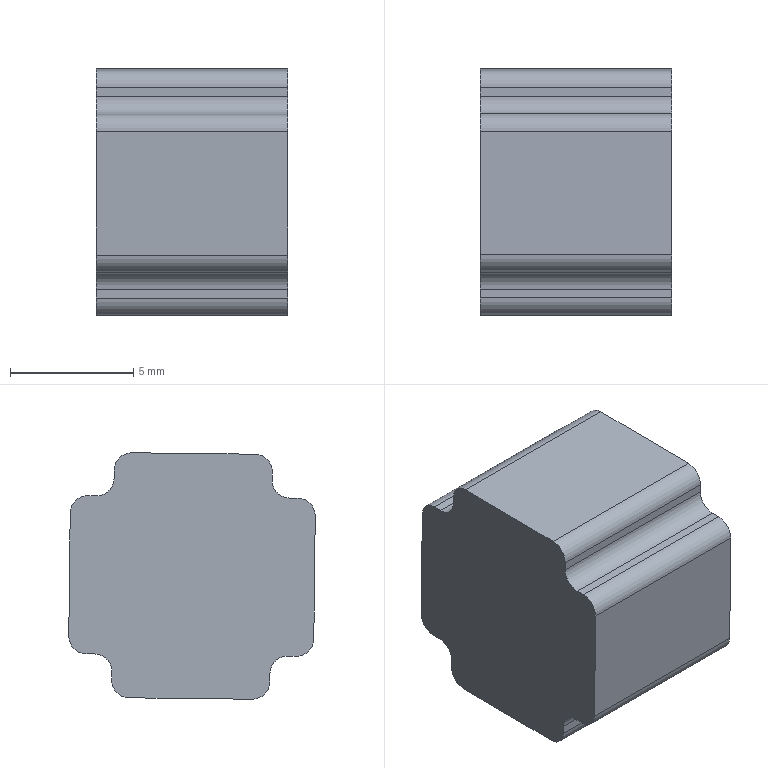Part | SolidWorks | features SplitBody 1 | 1 solid | 26 faces | box 7.744 x 9.983 x 9.983 mm | volume 663.797 mm3 | plane 14 | cylinder 12 | commonest cylinder face diameters 1.408 x12
STEP:
#1=CARTESIAN_POINT('',(576.371,440.454,-345.037));
#2=VERTEX_POINT('',#1);
#3=CARTESIAN_POINT('',(576.371,441.166,-345.733));
#4=VERTEX_POINT('',#3);
#5=CARTESIAN_POINT('',(576.371,441.158,-345.029));
#6=DIRECTION('',(1.,0.,0.));
#7=DIRECTION('',(0.,0.9999,0.01138));
#8=AXIS2_PLACEMENT_3D('',#5,#6,#7);
#9=CIRCLE('',#8,0.704);
#10=EDGE_CURVE('',#2,#4,#9,.T.);
#11=ORIENTED_EDGE('',*,*,#10,.T.);
#12=CARTESIAN_POINT('',(584.115,441.166,-345.733));
#13=VERTEX_POINT('',#12);
#14=CARTESIAN_POINT('',(584.115,441.166,-345.733));
#15=DIRECTION('',(-1.,0.,0.));
#16=VECTOR('',#15,1000.);
#17=LINE('',#14,#16);
#18=EDGE_CURVE('',#13,#4,#17,.T.);
#19=ORIENTED_EDGE('',*,*,#18,.F.);
#20=CARTESIAN_POINT('',(584.115,440.454,-345.037));
#21=VERTEX_POINT('',#20);
#22=CARTESIAN_POINT('',(584.115,441.158,-345.029));
#23=DIRECTION('',(1.,0.,0.));
#24=DIRECTION('',(0.,0.9999,0.01138));
#25=AXIS2_PLACEMENT_3D('',#22,#23,#24);
#26=CIRCLE('',#25,0.704);
#27=EDGE_CURVE('',#21,#13,#26,.T.);
#28=ORIENTED_EDGE('',*,*,#27,.F.);
#29=CARTESIAN_POINT('',(584.115,440.454,-345.037));
#30=DIRECTION('',(-1.,0.,0.));
#31=VECTOR('',#30,1000.);
#32=LINE('',#29,#31);
#33=EDGE_CURVE('',#21,#2,#32,.T.);
#34=ORIENTED_EDGE('',*,*,#33,.T.);
#35=EDGE_LOOP('',(#11,#19,#28,#34));
#36=FACE_OUTER_BOUND('',#35,.T.);
#37=CARTESIAN_POINT('',(584.115,441.158,-345.029));
#38=DIRECTION('',(-1.,0.,0.));
#39=DIRECTION('',(0.,-0.9999,-0.01138));
#40=AXIS2_PLACEMENT_3D('',#37,#38,#39);
#41=CYLINDRICAL_SURFACE('',#40,0.704);
#42=ADVANCED_FACE('',(#36),#41,.T.);
#43=CARTESIAN_POINT('',(576.371,441.518,-345.729));
#44=VERTEX_POINT('',#43);
#45=CARTESIAN_POINT('',(576.371,441.166,-345.733));
#46=DIRECTION('',(0.,0.9999,0.01138));
#47=VECTOR('',#46,1000.);
#48=LINE('',#45,#47);
#49=EDGE_CURVE('',#4,#44,#48,.T.);
#50=ORIENTED_EDGE('',*,*,#49,.T.);
#51=CARTESIAN_POINT('',(584.115,441.518,-345.729));
#52=VERTEX_POINT('',#51);
#53=CARTESIAN_POINT('',(584.115,441.518,-345.729));
#54=DIRECTION('',(-1.,0.,0.));
#55=VECTOR('',#54,1000.);
#56=LINE('',#53,#55);
#57=EDGE_CURVE('',#52,#44,#56,.T.);
#58=ORIENTED_EDGE('',*,*,#57,.F.);
#59=CARTESIAN_POINT('',(584.115,441.166,-345.733));
#60=DIRECTION('',(0.,0.9999,0.01138));
#61=VECTOR('',#60,1000.);
#62=LINE('',#59,#61);
#63=EDGE_CURVE('',#13,#52,#62,.T.);
#64=ORIENTED_EDGE('',*,*,#63,.F.);
#65=ORIENTED_EDGE('',*,*,#18,.T.);
#66=EDGE_LOOP('',(#50,#58,#64,#65));
#67=FACE_OUTER_BOUND('',#66,.T.);
#68=CARTESIAN_POINT('',(584.115,441.166,-345.733));
#69=DIRECTION('',(0.,-0.01138,0.9999));
#70=DIRECTION('',(1.,0.,0.));
#71=AXIS2_PLACEMENT_3D('',#68,#69,#70);
#72=PLANE('',#71);
#73=ADVANCED_FACE('',(#67),#72,.F.);
#74=CARTESIAN_POINT('',(576.371,442.23,-346.425));
#75=VERTEX_POINT('',#74);
#76=CARTESIAN_POINT('',(576.371,441.526,-346.433));
#77=DIRECTION('',(-1.,0.,0.));
#78=DIRECTION('',(0.,0.9999,0.01138));
#79=AXIS2_PLACEMENT_3D('',#76,#77,#78);
#80=CIRCLE('',#79,0.704);
#81=EDGE_CURVE('',#44,#75,#80,.T.);
#82=ORIENTED_EDGE('',*,*,#81,.T.);
#83=CARTESIAN_POINT('',(584.115,442.23,-346.425));
#84=VERTEX_POINT('',#83);
#85=CARTESIAN_POINT('',(584.115,442.23,-346.425));
#86=DIRECTION('',(-1.,0.,0.));
#87=VECTOR('',#86,1000.);
#88=LINE('',#85,#87);
#89=EDGE_CURVE('',#84,#75,#88,.T.);
#90=ORIENTED_EDGE('',*,*,#89,.F.);
#91=CARTESIAN_POINT('',(584.115,441.526,-346.433));
#92=DIRECTION('',(-1.,0.,0.));
#93=DIRECTION('',(0.,0.9999,0.01138));
#94=AXIS2_PLACEMENT_3D('',#91,#92,#93);
#95=CIRCLE('',#94,0.704);
#96=EDGE_CURVE('',#52,#84,#95,.T.);
#97=ORIENTED_EDGE('',*,*,#96,.F.);
#98=ORIENTED_EDGE('',*,*,#57,.T.);
#99=EDGE_LOOP('',(#82,#90,#97,#98));
#100=FACE_OUTER_BOUND('',#99,.T.);
#101=CARTESIAN_POINT('',(584.115,441.526,-346.433));
#102=DIRECTION('',(-1.,0.,0.));
#103=DIRECTION('',(0.,-0.9999,-0.01138));
#104=AXIS2_PLACEMENT_3D('',#101,#102,#103);
#105=CYLINDRICAL_SURFACE('',#104,0.704);
#106=ADVANCED_FACE('',(#100),#105,.F.);
#107=CARTESIAN_POINT('',(576.371,442.234,-346.777));
#108=VERTEX_POINT('',#107);
#109=CARTESIAN_POINT('',(576.371,442.23,-346.425));
#110=DIRECTION('',(0.,0.01138,-0.9999));
#111=VECTOR('',#110,1000.);
#112=LINE('',#109,#111);
#113=EDGE_CURVE('',#75,#108,#112,.T.);
#114=ORIENTED_EDGE('',*,*,#113,.T.);
#115=CARTESIAN_POINT('',(584.115,442.234,-346.777));
#116=VERTEX_POINT('',#115);
#117=CARTESIAN_POINT('',(584.115,442.234,-346.777));
#118=DIRECTION('',(-1.,0.,0.));
#119=VECTOR('',#118,1000.);
#120=LINE('',#117,#119);
#121=EDGE_CURVE('',#116,#108,#120,.T.);
#122=ORIENTED_EDGE('',*,*,#121,.F.);
#123=CARTESIAN_POINT('',(584.115,442.23,-346.425));
#124=DIRECTION('',(0.,0.01138,-0.9999));
#125=VECTOR('',#124,1000.);
#126=LINE('',#123,#125);
#127=EDGE_CURVE('',#84,#116,#126,.T.);
#128=ORIENTED_EDGE('',*,*,#127,.F.);
#129=ORIENTED_EDGE('',*,*,#89,.T.);
#130=EDGE_LOOP('',(#114,#122,#128,#129));
#131=FACE_OUTER_BOUND('',#130,.T.);
#132=CARTESIAN_POINT('',(584.115,442.23,-346.425));
#133=DIRECTION('',(0.,0.9999,0.01138));
#134=DIRECTION('',(-1.,0.,0.));
#135=AXIS2_PLACEMENT_3D('',#132,#133,#134);
#136=PLANE('',#135);
#137=ADVANCED_FACE('',(#131),#136,.F.);
#138=CARTESIAN_POINT('',(576.371,442.946,-347.473));
#139=VERTEX_POINT('',#138);
#140=CARTESIAN_POINT('',(576.371,442.938,-346.769));
#141=DIRECTION('',(1.,0.,0.));
#142=DIRECTION('',(0.,0.9999,0.01138));
#143=AXIS2_PLACEMENT_3D('',#140,#141,#142);
#144=CIRCLE('',#143,0.704);
#145=EDGE_CURVE('',#108,#139,#144,.T.);
#146=ORIENTED_EDGE('',*,*,#145,.T.);
#147=CARTESIAN_POINT('',(584.115,442.946,-347.473));
#148=VERTEX_POINT('',#147);
#149=CARTESIAN_POINT('',(584.115,442.946,-347.473));
#150=DIRECTION('',(-1.,0.,0.));
#151=VECTOR('',#150,1000.);
#152=LINE('',#149,#151);
#153=EDGE_CURVE('',#148,#139,#152,.T.);
#154=ORIENTED_EDGE('',*,*,#153,.F.);
#155=CARTESIAN_POINT('',(584.115,442.938,-346.769));
#156=DIRECTION('',(1.,0.,0.));
#157=DIRECTION('',(0.,0.9999,0.01138));
#158=AXIS2_PLACEMENT_3D('',#155,#156,#157);
#159=CIRCLE('',#158,0.704);
#160=EDGE_CURVE('',#116,#148,#159,.T.);
#161=ORIENTED_EDGE('',*,*,#160,.F.);
#162=ORIENTED_EDGE('',*,*,#121,.T.);
#163=EDGE_LOOP('',(#146,#154,#161,#162));
#164=FACE_OUTER_BOUND('',#163,.T.);
#165=CARTESIAN_POINT('',(584.115,442.938,-346.769));
#166=DIRECTION('',(-1.,0.,0.));
#167=DIRECTION('',(0.,-0.9999,-0.01138));
#168=AXIS2_PLACEMENT_3D('',#165,#166,#167);
#169=CYLINDRICAL_SURFACE('',#168,0.704);
#170=ADVANCED_FACE('',(#164),#169,.T.);
#171=CARTESIAN_POINT('',(576.371,447.944,-347.416));
#172=VERTEX_POINT('',#171);
#173=CARTESIAN_POINT('',(576.371,442.946,-347.473));
#174=DIRECTION('',(0.,0.9999,0.01138));
#175=VECTOR('',#174,1000.);
#176=LINE('',#173,#175);
#177=EDGE_CURVE('',#139,#172,#176,.T.);
#178=ORIENTED_EDGE('',*,*,#177,.T.);
#179=CARTESIAN_POINT('',(584.115,447.944,-347.416));
#180=VERTEX_POINT('',#179);
#181=CARTESIAN_POINT('',(584.115,447.944,-347.416));
#182=DIRECTION('',(-1.,0.,0.));
#183=VECTOR('',#182,1000.);
#184=LINE('',#181,#183);
#185=EDGE_CURVE('',#180,#172,#184,.T.);
#186=ORIENTED_EDGE('',*,*,#185,.F.);
#187=CARTESIAN_POINT('',(584.115,442.946,-347.473));
#188=DIRECTION('',(0.,0.9999,0.01138));
#189=VECTOR('',#188,1000.);
#190=LINE('',#187,#189);
#191=EDGE_CURVE('',#148,#180,#190,.T.);
#192=ORIENTED_EDGE('',*,*,#191,.F.);
#193=ORIENTED_EDGE('',*,*,#153,.T.);
#194=EDGE_LOOP('',(#178,#186,#192,#193));
#195=FACE_OUTER_BOUND('',#194,.T.);
#196=CARTESIAN_POINT('',(584.115,442.946,-347.473));
#197=DIRECTION('',(0.,-0.01138,0.9999));
#198=DIRECTION('',(1.,0.,0.));
#199=AXIS2_PLACEMENT_3D('',#196,#197,#198);
#200=PLANE('',#199);
#201=ADVANCED_FACE('',(#195),#200,.F.);
#202=CARTESIAN_POINT('',(576.371,448.64,-346.704));
#203=VERTEX_POINT('',#202);
#204=CARTESIAN_POINT('',(576.371,447.936,-346.712));
#205=DIRECTION('',(1.,0.,0.));
#206=DIRECTION('',(0.,0.9999,0.01138));
#207=AXIS2_PLACEMENT_3D('',#204,#205,#206);
#208=CIRCLE('',#207,0.704);
#209=EDGE_CURVE('',#172,#203,#208,.T.);
#210=ORIENTED_EDGE('',*,*,#209,.T.);
#211=CARTESIAN_POINT('',(584.115,448.64,-346.704));
#212=VERTEX_POINT('',#211);
#213=CARTESIAN_POINT('',(584.115,448.64,-346.704));
#214=DIRECTION('',(-1.,0.,0.));
#215=VECTOR('',#214,1000.);
#216=LINE('',#213,#215);
#217=EDGE_CURVE('',#212,#203,#216,.T.);
#218=ORIENTED_EDGE('',*,*,#217,.F.);
#219=CARTESIAN_POINT('',(584.115,447.936,-346.712));
#220=DIRECTION('',(1.,0.,0.));
#221=DIRECTION('',(0.,0.9999,0.01138));
#222=AXIS2_PLACEMENT_3D('',#219,#220,#221);
#223=CIRCLE('',#222,0.704);
#224=EDGE_CURVE('',#180,#212,#223,.T.);
#225=ORIENTED_EDGE('',*,*,#224,.F.);
#226=ORIENTED_EDGE('',*,*,#185,.T.);
#227=EDGE_LOOP('',(#210,#218,#225,#226));
#228=FACE_OUTER_BOUND('',#227,.T.);
#229=CARTESIAN_POINT('',(584.115,447.936,-346.712));
#230=DIRECTION('',(-1.,0.,0.));
#231=DIRECTION('',(0.,-0.9999,-0.01138));
#232=AXIS2_PLACEMENT_3D('',#229,#230,#231);
#233=CYLINDRICAL_SURFACE('',#232,0.704);
#234=ADVANCED_FACE('',(#228),#233,.T.);
#235=CARTESIAN_POINT('',(576.371,448.636,-346.352));
#236=VERTEX_POINT('',#235);
#237=CARTESIAN_POINT('',(576.371,448.64,-346.704));
#238=DIRECTION('',(0.,-0.01138,0.9999));
#239=VECTOR('',#238,1000.);
#240=LINE('',#237,#239);
#241=EDGE_CURVE('',#203,#236,#240,.T.);
#242=ORIENTED_EDGE('',*,*,#241,.T.);
#243=CARTESIAN_POINT('',(584.115,448.636,-346.352));
#244=VERTEX_POINT('',#243);
#245=CARTESIAN_POINT('',(584.115,448.636,-346.352));
#246=DIRECTION('',(-1.,0.,0.));
#247=VECTOR('',#246,1000.);
#248=LINE('',#245,#247);
#249=EDGE_CURVE('',#244,#236,#248,.T.);
#250=ORIENTED_EDGE('',*,*,#249,.F.);
#251=CARTESIAN_POINT('',(584.115,448.64,-346.704));
#252=DIRECTION('',(0.,-0.01138,0.9999));
#253=VECTOR('',#252,1000.);
#254=LINE('',#251,#253);
#255=EDGE_CURVE('',#212,#244,#254,.T.);
#256=ORIENTED_EDGE('',*,*,#255,.F.);
#257=ORIENTED_EDGE('',*,*,#217,.T.);
#258=EDGE_LOOP('',(#242,#250,#256,#257));
#259=FACE_OUTER_BOUND('',#258,.T.);
#260=CARTESIAN_POINT('',(584.115,448.64,-346.704));
#261=DIRECTION('',(0.,-0.9999,-0.01138));
#262=DIRECTION('',(1.,0.,0.));
#263=AXIS2_PLACEMENT_3D('',#260,#261,#262);
#264=PLANE('',#263);
#265=ADVANCED_FACE('',(#259),#264,.F.);
#266=CARTESIAN_POINT('',(576.371,449.331,-345.64));
#267=VERTEX_POINT('',#266);
#268=CARTESIAN_POINT('',(576.371,449.339,-346.344));
#269=DIRECTION('',(-1.,0.,0.));
#270=DIRECTION('',(0.,0.9999,0.01138));
#271=AXIS2_PLACEMENT_3D('',#268,#269,#270);
#272=CIRCLE('',#271,0.704);
#273=EDGE_CURVE('',#236,#267,#272,.T.);
#274=ORIENTED_EDGE('',*,*,#273,.T.);
#275=CARTESIAN_POINT('',(584.115,449.331,-345.64));
#276=VERTEX_POINT('',#275);
#277=CARTESIAN_POINT('',(584.115,449.331,-345.64));
#278=DIRECTION('',(-1.,0.,0.));
#279=VECTOR('',#278,1000.);
#280=LINE('',#277,#279);
#281=EDGE_CURVE('',#276,#267,#280,.T.);
#282=ORIENTED_EDGE('',*,*,#281,.F.);
#283=CARTESIAN_POINT('',(584.115,449.339,-346.344));
#284=DIRECTION('',(-1.,0.,0.));
#285=DIRECTION('',(0.,0.9999,0.01138));
#286=AXIS2_PLACEMENT_3D('',#283,#284,#285);
#287=CIRCLE('',#286,0.704);
#288=EDGE_CURVE('',#244,#276,#287,.T.);
#289=ORIENTED_EDGE('',*,*,#288,.F.);
#290=ORIENTED_EDGE('',*,*,#249,.T.);
#291=EDGE_LOOP('',(#274,#282,#289,#290));
#292=FACE_OUTER_BOUND('',#291,.T.);
#293=CARTESIAN_POINT('',(584.115,449.339,-346.344));
#294=DIRECTION('',(-1.,0.,0.));
#295=DIRECTION('',(0.,-0.9999,-0.01138));
#296=AXIS2_PLACEMENT_3D('',#293,#294,#295);
#297=CYLINDRICAL_SURFACE('',#296,0.704);
#298=ADVANCED_FACE('',(#292),#297,.F.);
#299=CARTESIAN_POINT('',(576.371,449.683,-345.636));
#300=VERTEX_POINT('',#299);
#301=CARTESIAN_POINT('',(576.371,449.331,-345.64));
#302=DIRECTION('',(0.,0.9999,0.01138));
#303=VECTOR('',#302,1000.);
#304=LINE('',#301,#303);
#305=EDGE_CURVE('',#267,#300,#304,.T.);
#306=ORIENTED_EDGE('',*,*,#305,.T.);
#307=CARTESIAN_POINT('',(584.115,449.683,-345.636));
#308=VERTEX_POINT('',#307);
#309=CARTESIAN_POINT('',(584.115,449.683,-345.636));
#310=DIRECTION('',(-1.,0.,0.));
#311=VECTOR('',#310,1000.);
#312=LINE('',#309,#311);
#313=EDGE_CURVE('',#308,#300,#312,.T.);
#314=ORIENTED_EDGE('',*,*,#313,.F.);
#315=CARTESIAN_POINT('',(584.115,449.331,-345.64));
#316=DIRECTION('',(0.,0.9999,0.01138));
#317=VECTOR('',#316,1000.);
#318=LINE('',#315,#317);
#319=EDGE_CURVE('',#276,#308,#318,.T.);
#320=ORIENTED_EDGE('',*,*,#319,.F.);
#321=ORIENTED_EDGE('',*,*,#281,.T.);
#322=EDGE_LOOP('',(#306,#314,#320,#321));
#323=FACE_OUTER_BOUND('',#322,.T.);
#324=CARTESIAN_POINT('',(584.115,449.331,-345.64));
#325=DIRECTION('',(0.,-0.01138,0.9999));
#326=DIRECTION('',(1.,0.,0.));
#327=AXIS2_PLACEMENT_3D('',#324,#325,#326);
#328=PLANE('',#327);
#329=ADVANCED_FACE('',(#323),#328,.F.);
#330=CARTESIAN_POINT('',(576.371,450.379,-344.924));
#331=VERTEX_POINT('',#330);
#332=CARTESIAN_POINT('',(576.371,449.675,-344.932));
#333=DIRECTION('',(1.,0.,0.));
#334=DIRECTION('',(0.,0.9999,0.01138));
#335=AXIS2_PLACEMENT_3D('',#332,#333,#334);
#336=CIRCLE('',#335,0.704);
#337=EDGE_CURVE('',#300,#331,#336,.T.);
#338=ORIENTED_EDGE('',*,*,#337,.T.);
#339=CARTESIAN_POINT('',(584.115,450.379,-344.924));
#340=VERTEX_POINT('',#339);
#341=CARTESIAN_POINT('',(584.115,450.379,-344.924));
#342=DIRECTION('',(-1.,0.,0.));
#343=VECTOR('',#342,1000.);
#344=LINE('',#341,#343);
#345=EDGE_CURVE('',#340,#331,#344,.T.);
#346=ORIENTED_EDGE('',*,*,#345,.F.);
#347=CARTESIAN_POINT('',(584.115,449.675,-344.932));
#348=DIRECTION('',(1.,0.,0.));
#349=DIRECTION('',(0.,0.9999,0.01138));
#350=AXIS2_PLACEMENT_3D('',#347,#348,#349);
#351=CIRCLE('',#350,0.704);
#352=EDGE_CURVE('',#308,#340,#351,.T.);
#353=ORIENTED_EDGE('',*,*,#352,.F.);
#354=ORIENTED_EDGE('',*,*,#313,.T.);
#355=EDGE_LOOP('',(#338,#346,#353,#354));
#356=FACE_OUTER_BOUND('',#355,.T.);
#357=CARTESIAN_POINT('',(584.115,449.675,-344.932));
#358=DIRECTION('',(-1.,0.,0.));
#359=DIRECTION('',(0.,-0.9999,-0.01138));
#360=AXIS2_PLACEMENT_3D('',#357,#358,#359);
#361=CYLINDRICAL_SURFACE('',#360,0.704);
#362=ADVANCED_FACE('',(#356),#361,.T.);
#363=CARTESIAN_POINT('',(576.371,450.323,-339.926));
#364=VERTEX_POINT('',#363);
#365=CARTESIAN_POINT('',(576.371,450.379,-344.924));
#366=DIRECTION('',(0.,-0.01138,0.9999));
#367=VECTOR('',#366,1000.);
#368=LINE('',#365,#367);
#369=EDGE_CURVE('',#331,#364,#368,.T.);
#370=ORIENTED_EDGE('',*,*,#369,.T.);
#371=CARTESIAN_POINT('',(584.115,450.323,-339.926));
#372=VERTEX_POINT('',#371);
#373=CARTESIAN_POINT('',(584.115,450.323,-339.926));
#374=DIRECTION('',(-1.,0.,0.));
#375=VECTOR('',#374,1000.);
#376=LINE('',#373,#375);
#377=EDGE_CURVE('',#372,#364,#376,.T.);
#378=ORIENTED_EDGE('',*,*,#377,.F.);
#379=CARTESIAN_POINT('',(584.115,450.379,-344.924));
#380=DIRECTION('',(0.,-0.01138,0.9999));
#381=VECTOR('',#380,1000.);
#382=LINE('',#379,#381);
#383=EDGE_CURVE('',#340,#372,#382,.T.);
#384=ORIENTED_EDGE('',*,*,#383,.F.);
#385=ORIENTED_EDGE('',*,*,#345,.T.);
#386=EDGE_LOOP('',(#370,#378,#384,#385));
#387=FACE_OUTER_BOUND('',#386,.T.);
#388=CARTESIAN_POINT('',(584.115,450.379,-344.924));
#389=DIRECTION('',(0.,-0.9999,-0.01138));
#390=DIRECTION('',(0.,0.01138,-0.9999));
#391=AXIS2_PLACEMENT_3D('',#388,#389,#390);
#392=PLANE('',#391);
#393=ADVANCED_FACE('',(#387),#392,.F.);
#394=CARTESIAN_POINT('',(576.371,449.611,-339.23));
#395=VERTEX_POINT('',#394);
#396=CARTESIAN_POINT('',(576.371,449.619,-339.934));
#397=DIRECTION('',(1.,0.,0.));
#398=DIRECTION('',(0.,0.9999,0.01138));
#399=AXIS2_PLACEMENT_3D('',#396,#397,#398);
#400=CIRCLE('',#399,0.704);
#401=EDGE_CURVE('',#364,#395,#400,.T.);
#402=ORIENTED_EDGE('',*,*,#401,.T.);
#403=CARTESIAN_POINT('',(584.115,449.611,-339.23));
#404=VERTEX_POINT('',#403);
#405=CARTESIAN_POINT('',(584.115,449.611,-339.23));
#406=DIRECTION('',(-1.,0.,0.));
#407=VECTOR('',#406,1000.);
#408=LINE('',#405,#407);
#409=EDGE_CURVE('',#404,#395,#408,.T.);
#410=ORIENTED_EDGE('',*,*,#409,.F.);
#411=CARTESIAN_POINT('',(584.115,449.619,-339.934));
#412=DIRECTION('',(1.,0.,0.));
#413=DIRECTION('',(0.,0.9999,0.01138));
#414=AXIS2_PLACEMENT_3D('',#411,#412,#413);
#415=CIRCLE('',#414,0.704);
#416=EDGE_CURVE('',#372,#404,#415,.T.);
#417=ORIENTED_EDGE('',*,*,#416,.F.);
#418=ORIENTED_EDGE('',*,*,#377,.T.);
#419=EDGE_LOOP('',(#402,#410,#417,#418));
#420=FACE_OUTER_BOUND('',#419,.T.);
#421=CARTESIAN_POINT('',(584.115,449.619,-339.934));
#422=DIRECTION('',(-1.,0.,0.));
#423=DIRECTION('',(0.,-0.9999,-0.01138));
#424=AXIS2_PLACEMENT_3D('',#421,#422,#423);
#425=CYLINDRICAL_SURFACE('',#424,0.704);
#426=ADVANCED_FACE('',(#420),#425,.T.);
#427=CARTESIAN_POINT('',(576.371,449.259,-339.234));
#428=VERTEX_POINT('',#427);
#429=CARTESIAN_POINT('',(576.371,449.611,-339.23));
#430=DIRECTION('',(0.,-0.9999,-0.01138));
#431=VECTOR('',#430,1000.);
#432=LINE('',#429,#431);
#433=EDGE_CURVE('',#395,#428,#432,.T.);
#434=ORIENTED_EDGE('',*,*,#433,.T.);
#435=CARTESIAN_POINT('',(584.115,449.259,-339.234));
#436=VERTEX_POINT('',#435);
#437=CARTESIAN_POINT('',(584.115,449.259,-339.234));
#438=DIRECTION('',(-1.,0.,0.));
#439=VECTOR('',#438,1000.);
#440=LINE('',#437,#439);
#441=EDGE_CURVE('',#436,#428,#440,.T.);
#442=ORIENTED_EDGE('',*,*,#441,.F.);
#443=CARTESIAN_POINT('',(584.115,449.611,-339.23));
#444=DIRECTION('',(0.,-0.9999,-0.01138));
#445=VECTOR('',#444,1000.);
#446=LINE('',#443,#445);
#447=EDGE_CURVE('',#404,#436,#446,.T.);
#448=ORIENTED_EDGE('',*,*,#447,.F.);
#449=ORIENTED_EDGE('',*,*,#409,.T.);
#450=EDGE_LOOP('',(#434,#442,#448,#449));
#451=FACE_OUTER_BOUND('',#450,.T.);
#452=CARTESIAN_POINT('',(584.115,449.611,-339.23));
#453=DIRECTION('',(0.,0.01138,-0.9999));
#454=DIRECTION('',(-1.,0.,0.));
#455=AXIS2_PLACEMENT_3D('',#452,#453,#454);
#456=PLANE('',#455);
#457=ADVANCED_FACE('',(#451),#456,.F.);
#458=CARTESIAN_POINT('',(576.371,448.547,-338.538));
#459=VERTEX_POINT('',#458);
#460=CARTESIAN_POINT('',(576.371,449.251,-338.53));
#461=DIRECTION('',(-1.,0.,0.));
#462=DIRECTION('',(0.,0.9999,0.01138));
#463=AXIS2_PLACEMENT_3D('',#460,#461,#462);
#464=CIRCLE('',#463,0.704);
#465=EDGE_CURVE('',#428,#459,#464,.T.);
#466=ORIENTED_EDGE('',*,*,#465,.T.);
#467=CARTESIAN_POINT('',(584.115,448.547,-338.538));
#468=VERTEX_POINT('',#467);
#469=CARTESIAN_POINT('',(584.115,448.547,-338.538));
#470=DIRECTION('',(-1.,0.,0.));
#471=VECTOR('',#470,1000.);
#472=LINE('',#469,#471);
#473=EDGE_CURVE('',#468,#459,#472,.T.);
#474=ORIENTED_EDGE('',*,*,#473,.F.);
#475=CARTESIAN_POINT('',(584.115,449.251,-338.53));
#476=DIRECTION('',(-1.,0.,0.));
#477=DIRECTION('',(0.,0.9999,0.01138));
#478=AXIS2_PLACEMENT_3D('',#475,#476,#477);
#479=CIRCLE('',#478,0.704);
#480=EDGE_CURVE('',#436,#468,#479,.T.);
#481=ORIENTED_EDGE('',*,*,#480,.F.);
#482=ORIENTED_EDGE('',*,*,#441,.T.);
#483=EDGE_LOOP('',(#466,#474,#481,#482));
#484=FACE_OUTER_BOUND('',#483,.T.);
#485=CARTESIAN_POINT('',(584.115,449.251,-338.53));
#486=DIRECTION('',(-1.,0.,0.));
#487=DIRECTION('',(0.,-0.9999,-0.01138));
#488=AXIS2_PLACEMENT_3D('',#485,#486,#487);
#489=CYLINDRICAL_SURFACE('',#488,0.704);
#490=ADVANCED_FACE('',(#484),#489,.F.);
#491=CARTESIAN_POINT('',(576.371,448.543,-338.186));
#492=VERTEX_POINT('',#491);
#493=CARTESIAN_POINT('',(576.371,448.547,-338.538));
#494=DIRECTION('',(0.,-0.01138,0.9999));
#495=VECTOR('',#494,1000.);
#496=LINE('',#493,#495);
#497=EDGE_CURVE('',#459,#492,#496,.T.);
#498=ORIENTED_EDGE('',*,*,#497,.T.);
#499=CARTESIAN_POINT('',(584.115,448.543,-338.186));
#500=VERTEX_POINT('',#499);
#501=CARTESIAN_POINT('',(584.115,448.543,-338.186));
#502=DIRECTION('',(-1.,0.,0.));
#503=VECTOR('',#502,1000.);
#504=LINE('',#501,#503);
#505=EDGE_CURVE('',#500,#492,#504,.T.);
#506=ORIENTED_EDGE('',*,*,#505,.F.);
#507=CARTESIAN_POINT('',(584.115,448.547,-338.538));
#508=DIRECTION('',(0.,-0.01138,0.9999));
#509=VECTOR('',#508,1000.);
#510=LINE('',#507,#509);
#511=EDGE_CURVE('',#468,#500,#510,.T.);
#512=ORIENTED_EDGE('',*,*,#511,.F.);
#513=ORIENTED_EDGE('',*,*,#473,.T.);
#514=EDGE_LOOP('',(#498,#506,#512,#513));
#515=FACE_OUTER_BOUND('',#514,.T.);
#516=CARTESIAN_POINT('',(584.115,448.547,-338.538));
#517=DIRECTION('',(0.,-0.9999,-0.01138));
#518=DIRECTION('',(1.,0.,0.));
#519=AXIS2_PLACEMENT_3D('',#516,#517,#518);
#520=PLANE('',#519);
#521=ADVANCED_FACE('',(#515),#520,.F.);
#522=CARTESIAN_POINT('',(576.371,447.831,-337.49));
#523=VERTEX_POINT('',#522);
#524=CARTESIAN_POINT('',(576.371,447.839,-338.194));
#525=DIRECTION('',(1.,0.,0.));
#526=DIRECTION('',(0.,0.9999,0.01138));
#527=AXIS2_PLACEMENT_3D('',#524,#525,#526);
#528=CIRCLE('',#527,0.704);
#529=EDGE_CURVE('',#492,#523,#528,.T.);
#530=ORIENTED_EDGE('',*,*,#529,.T.);
#531=CARTESIAN_POINT('',(584.115,447.831,-337.49));
#532=VERTEX_POINT('',#531);
#533=CARTESIAN_POINT('',(584.115,447.831,-337.49));
#534=DIRECTION('',(-1.,0.,0.));
#535=VECTOR('',#534,1000.);
#536=LINE('',#533,#535);
#537=EDGE_CURVE('',#532,#523,#536,.T.);
#538=ORIENTED_EDGE('',*,*,#537,.F.);
#539=CARTESIAN_POINT('',(584.115,447.839,-338.194));
#540=DIRECTION('',(1.,0.,0.));
#541=DIRECTION('',(0.,0.9999,0.01138));
#542=AXIS2_PLACEMENT_3D('',#539,#540,#541);
#543=CIRCLE('',#542,0.704);
#544=EDGE_CURVE('',#500,#532,#543,.T.);
#545=ORIENTED_EDGE('',*,*,#544,.F.);
#546=ORIENTED_EDGE('',*,*,#505,.T.);
#547=EDGE_LOOP('',(#530,#538,#545,#546));
#548=FACE_OUTER_BOUND('',#547,.T.);
#549=CARTESIAN_POINT('',(584.115,447.839,-338.194));
#550=DIRECTION('',(-1.,0.,0.));
#551=DIRECTION('',(0.,-0.9999,-0.01138));
#552=AXIS2_PLACEMENT_3D('',#549,#550,#551);
#553=CYLINDRICAL_SURFACE('',#552,0.704);
#554=ADVANCED_FACE('',(#548),#553,.T.);
#555=CARTESIAN_POINT('',(576.371,442.833,-337.547));
#556=VERTEX_POINT('',#555);
#557=CARTESIAN_POINT('',(576.371,447.831,-337.49));
#558=DIRECTION('',(0.,-0.9999,-0.01138));
#559=VECTOR('',#558,1000.);
#560=LINE('',#557,#559);
#561=EDGE_CURVE('',#523,#556,#560,.T.);
#562=ORIENTED_EDGE('',*,*,#561,.T.);
#563=CARTESIAN_POINT('',(584.115,442.833,-337.547));
#564=VERTEX_POINT('',#563);
#565=CARTESIAN_POINT('',(584.115,442.833,-337.547));
#566=DIRECTION('',(-1.,0.,0.));
#567=VECTOR('',#566,1000.);
#568=LINE('',#565,#567);
#569=EDGE_CURVE('',#564,#556,#568,.T.);
#570=ORIENTED_EDGE('',*,*,#569,.F.);
#571=CARTESIAN_POINT('',(584.115,447.831,-337.49));
#572=DIRECTION('',(0.,-0.9999,-0.01138));
#573=VECTOR('',#572,1000.);
#574=LINE('',#571,#573);
#575=EDGE_CURVE('',#532,#564,#574,.T.);
#576=ORIENTED_EDGE('',*,*,#575,.F.);
#577=ORIENTED_EDGE('',*,*,#537,.T.);
#578=EDGE_LOOP('',(#562,#570,#576,#577));
#579=FACE_OUTER_BOUND('',#578,.T.);
#580=CARTESIAN_POINT('',(584.115,447.831,-337.49));
#581=DIRECTION('',(0.,0.01138,-0.9999));
#582=DIRECTION('',(-1.,0.,0.));
#583=AXIS2_PLACEMENT_3D('',#580,#581,#582);
#584=PLANE('',#583);
#585=ADVANCED_FACE('',(#579),#584,.F.);
#586=CARTESIAN_POINT('',(576.371,442.137,-338.259));
#587=VERTEX_POINT('',#586);
#588=CARTESIAN_POINT('',(576.371,442.841,-338.251));
#589=DIRECTION('',(1.,0.,0.));
#590=DIRECTION('',(0.,0.9999,0.01138));
#591=AXIS2_PLACEMENT_3D('',#588,#589,#590);
#592=CIRCLE('',#591,0.704);
#593=EDGE_CURVE('',#556,#587,#592,.T.);
#594=ORIENTED_EDGE('',*,*,#593,.T.);
#595=CARTESIAN_POINT('',(584.115,442.137,-338.259));
#596=VERTEX_POINT('',#595);
#597=CARTESIAN_POINT('',(584.115,442.137,-338.259));
#598=DIRECTION('',(-1.,0.,0.));
#599=VECTOR('',#598,1000.);
#600=LINE('',#597,#599);
#601=EDGE_CURVE('',#596,#587,#600,.T.);
#602=ORIENTED_EDGE('',*,*,#601,.F.);
#603=CARTESIAN_POINT('',(584.115,442.841,-338.251));
#604=DIRECTION('',(1.,0.,0.));
#605=DIRECTION('',(0.,0.9999,0.01138));
#606=AXIS2_PLACEMENT_3D('',#603,#604,#605);
#607=CIRCLE('',#606,0.704);
#608=EDGE_CURVE('',#564,#596,#607,.T.);
#609=ORIENTED_EDGE('',*,*,#608,.F.);
#610=ORIENTED_EDGE('',*,*,#569,.T.);
#611=EDGE_LOOP('',(#594,#602,#609,#610));
#612=FACE_OUTER_BOUND('',#611,.T.);
#613=CARTESIAN_POINT('',(584.115,442.841,-338.251));
#614=DIRECTION('',(-1.,0.,0.));
#615=DIRECTION('',(0.,-0.9999,-0.01138));
#616=AXIS2_PLACEMENT_3D('',#613,#614,#615);
#617=CYLINDRICAL_SURFACE('',#616,0.704);
#618=ADVANCED_FACE('',(#612),#617,.T.);
#619=CARTESIAN_POINT('',(576.371,442.141,-338.611));
#620=VERTEX_POINT('',#619);
#621=CARTESIAN_POINT('',(576.371,442.137,-338.259));
#622=DIRECTION('',(0.,0.01138,-0.9999));
#623=VECTOR('',#622,1000.);
#624=LINE('',#621,#623);
#625=EDGE_CURVE('',#587,#620,#624,.T.);
#626=ORIENTED_EDGE('',*,*,#625,.T.);
#627=CARTESIAN_POINT('',(584.115,442.141,-338.611));
#628=VERTEX_POINT('',#627);
#629=CARTESIAN_POINT('',(584.115,442.141,-338.611));
#630=DIRECTION('',(-1.,0.,0.));
#631=VECTOR('',#630,1000.);
#632=LINE('',#629,#631);
#633=EDGE_CURVE('',#628,#620,#632,.T.);
#634=ORIENTED_EDGE('',*,*,#633,.F.);
#635=CARTESIAN_POINT('',(584.115,442.137,-338.259));
#636=DIRECTION('',(0.,0.01138,-0.9999));
#637=VECTOR('',#636,1000.);
#638=LINE('',#635,#637);
#639=EDGE_CURVE('',#596,#628,#638,.T.);
#640=ORIENTED_EDGE('',*,*,#639,.F.);
#641=ORIENTED_EDGE('',*,*,#601,.T.);
#642=EDGE_LOOP('',(#626,#634,#640,#641));
#643=FACE_OUTER_BOUND('',#642,.T.);
#644=CARTESIAN_POINT('',(584.115,442.137,-338.259));
#645=DIRECTION('',(0.,0.9999,0.01138));
#646=DIRECTION('',(-1.,0.,0.));
#647=AXIS2_PLACEMENT_3D('',#644,#645,#646);
#648=PLANE('',#647);
#649=ADVANCED_FACE('',(#643),#648,.F.);
#650=CARTESIAN_POINT('',(576.371,441.445,-339.323));
#651=VERTEX_POINT('',#650);
#652=CARTESIAN_POINT('',(576.371,441.437,-338.619));
#653=DIRECTION('',(-1.,0.,0.));
#654=DIRECTION('',(0.,0.9999,0.01138));
#655=AXIS2_PLACEMENT_3D('',#652,#653,#654);
#656=CIRCLE('',#655,0.704);
#657=EDGE_CURVE('',#620,#651,#656,.T.);
#658=ORIENTED_EDGE('',*,*,#657,.T.);
#659=CARTESIAN_POINT('',(584.115,441.445,-339.323));
#660=VERTEX_POINT('',#659);
#661=CARTESIAN_POINT('',(584.115,441.445,-339.323));
#662=DIRECTION('',(-1.,0.,0.));
#663=VECTOR('',#662,1000.);
#664=LINE('',#661,#663);
#665=EDGE_CURVE('',#660,#651,#664,.T.);
#666=ORIENTED_EDGE('',*,*,#665,.F.);
#667=CARTESIAN_POINT('',(584.115,441.437,-338.619));
#668=DIRECTION('',(-1.,0.,0.));
#669=DIRECTION('',(0.,0.9999,0.01138));
#670=AXIS2_PLACEMENT_3D('',#667,#668,#669);
#671=CIRCLE('',#670,0.704);
#672=EDGE_CURVE('',#628,#660,#671,.T.);
#673=ORIENTED_EDGE('',*,*,#672,.F.);
#674=ORIENTED_EDGE('',*,*,#633,.T.);
#675=EDGE_LOOP('',(#658,#666,#673,#674));
#676=FACE_OUTER_BOUND('',#675,.T.);
#677=CARTESIAN_POINT('',(584.115,441.437,-338.619));
#678=DIRECTION('',(-1.,0.,0.));
#679=DIRECTION('',(0.,-0.9999,-0.01138));
#680=AXIS2_PLACEMENT_3D('',#677,#678,#679);
#681=CYLINDRICAL_SURFACE('',#680,0.704);
#682=ADVANCED_FACE('',(#676),#681,.F.);
#683=CARTESIAN_POINT('',(576.371,441.093,-339.327));
#684=VERTEX_POINT('',#683);
#685=CARTESIAN_POINT('',(576.371,441.445,-339.323));
#686=DIRECTION('',(0.,-0.9999,-0.01138));
#687=VECTOR('',#686,1000.);
#688=LINE('',#685,#687);
#689=EDGE_CURVE('',#651,#684,#688,.T.);
#690=ORIENTED_EDGE('',*,*,#689,.T.);
#691=CARTESIAN_POINT('',(584.115,441.093,-339.327));
#692=VERTEX_POINT('',#691);
#693=CARTESIAN_POINT('',(584.115,441.093,-339.327));
#694=DIRECTION('',(-1.,0.,0.));
#695=VECTOR('',#694,1000.);
#696=LINE('',#693,#695);
#697=EDGE_CURVE('',#692,#684,#696,.T.);
#698=ORIENTED_EDGE('',*,*,#697,.F.);
#699=CARTESIAN_POINT('',(584.115,441.445,-339.323));
#700=DIRECTION('',(0.,-0.9999,-0.01138));
#701=VECTOR('',#700,1000.);
#702=LINE('',#699,#701);
#703=EDGE_CURVE('',#660,#692,#702,.T.);
#704=ORIENTED_EDGE('',*,*,#703,.F.);
#705=ORIENTED_EDGE('',*,*,#665,.T.);
#706=EDGE_LOOP('',(#690,#698,#704,#705));
#707=FACE_OUTER_BOUND('',#706,.T.);
#708=CARTESIAN_POINT('',(584.115,441.445,-339.323));
#709=DIRECTION('',(0.,0.01138,-0.9999));
#710=DIRECTION('',(-1.,0.,0.));
#711=AXIS2_PLACEMENT_3D('',#708,#709,#710);
#712=PLANE('',#711);
#713=ADVANCED_FACE('',(#707),#712,.F.);
#714=CARTESIAN_POINT('',(576.371,440.397,-340.039));
#715=VERTEX_POINT('',#714);
#716=CARTESIAN_POINT('',(576.371,441.101,-340.031));
#717=DIRECTION('',(1.,0.,0.));
#718=DIRECTION('',(0.,0.9999,0.01138));
#719=AXIS2_PLACEMENT_3D('',#716,#717,#718);
#720=CIRCLE('',#719,0.704);
#721=EDGE_CURVE('',#684,#715,#720,.T.);
#722=ORIENTED_EDGE('',*,*,#721,.T.);
#723=CARTESIAN_POINT('',(584.115,440.397,-340.039));
#724=VERTEX_POINT('',#723);
#725=CARTESIAN_POINT('',(584.115,440.397,-340.039));
#726=DIRECTION('',(-1.,0.,0.));
#727=VECTOR('',#726,1000.);
#728=LINE('',#725,#727);
#729=EDGE_CURVE('',#724,#715,#728,.T.);
#730=ORIENTED_EDGE('',*,*,#729,.F.);
#731=CARTESIAN_POINT('',(584.115,441.101,-340.031));
#732=DIRECTION('',(1.,0.,0.));
#733=DIRECTION('',(0.,0.9999,0.01138));
#734=AXIS2_PLACEMENT_3D('',#731,#732,#733);
#735=CIRCLE('',#734,0.704);
#736=EDGE_CURVE('',#692,#724,#735,.T.);
#737=ORIENTED_EDGE('',*,*,#736,.F.);
#738=ORIENTED_EDGE('',*,*,#697,.T.);
#739=EDGE_LOOP('',(#722,#730,#737,#738));
#740=FACE_OUTER_BOUND('',#739,.T.);
#741=CARTESIAN_POINT('',(584.115,441.101,-340.031));
#742=DIRECTION('',(-1.,0.,0.));
#743=DIRECTION('',(0.,-0.9999,-0.01138));
#744=AXIS2_PLACEMENT_3D('',#741,#742,#743);
#745=CYLINDRICAL_SURFACE('',#744,0.704);
#746=ADVANCED_FACE('',(#740),#745,.T.);
#747=CARTESIAN_POINT('',(576.371,440.397,-340.039));
#748=DIRECTION('',(0.,0.01138,-0.9999));
#749=VECTOR('',#748,1000.);
#750=LINE('',#747,#749);
#751=EDGE_CURVE('',#715,#2,#750,.T.);
#752=ORIENTED_EDGE('',*,*,#751,.T.);
#753=ORIENTED_EDGE('',*,*,#33,.F.);
#754=CARTESIAN_POINT('',(584.115,440.397,-340.039));
#755=DIRECTION('',(0.,0.01138,-0.9999));
#756=VECTOR('',#755,1000.);
#757=LINE('',#754,#756);
#758=EDGE_CURVE('',#724,#21,#757,.T.);
#759=ORIENTED_EDGE('',*,*,#758,.F.);
#760=ORIENTED_EDGE('',*,*,#729,.T.);
#761=EDGE_LOOP('',(#752,#753,#759,#760));
#762=FACE_OUTER_BOUND('',#761,.T.);
#763=CARTESIAN_POINT('',(584.115,440.397,-340.039));
#764=DIRECTION('',(0.,0.9999,0.01138));
#765=DIRECTION('',(-1.,0.,0.));
#766=AXIS2_PLACEMENT_3D('',#763,#764,#765);
#767=PLANE('',#766);
#768=ADVANCED_FACE('',(#762),#767,.F.);
#769=ORIENTED_EDGE('',*,*,#27,.T.);
#770=ORIENTED_EDGE('',*,*,#63,.T.);
#771=ORIENTED_EDGE('',*,*,#96,.T.);
#772=ORIENTED_EDGE('',*,*,#127,.T.);
#773=ORIENTED_EDGE('',*,*,#160,.T.);
#774=ORIENTED_EDGE('',*,*,#191,.T.);
#775=ORIENTED_EDGE('',*,*,#224,.T.);
#776=ORIENTED_EDGE('',*,*,#255,.T.);
#777=ORIENTED_EDGE('',*,*,#288,.T.);
#778=ORIENTED_EDGE('',*,*,#319,.T.);
#779=ORIENTED_EDGE('',*,*,#352,.T.);
#780=ORIENTED_EDGE('',*,*,#383,.T.);
#781=ORIENTED_EDGE('',*,*,#416,.T.);
#782=ORIENTED_EDGE('',*,*,#447,.T.);
#783=ORIENTED_EDGE('',*,*,#480,.T.);
#784=ORIENTED_EDGE('',*,*,#511,.T.);
#785=ORIENTED_EDGE('',*,*,#544,.T.);
#786=ORIENTED_EDGE('',*,*,#575,.T.);
#787=ORIENTED_EDGE('',*,*,#608,.T.);
#788=ORIENTED_EDGE('',*,*,#639,.T.);
#789=ORIENTED_EDGE('',*,*,#672,.T.);
#790=ORIENTED_EDGE('',*,*,#703,.T.);
#791=ORIENTED_EDGE('',*,*,#736,.T.);
#792=ORIENTED_EDGE('',*,*,#758,.T.);
#793=EDGE_LOOP('',(#769,#770,#771,#772,#773,#774,#775,#776,#777,#778,#779,#780,#781,#782,#783,#784,#785,#786,#787,#788,#789,#790,#791,#792));
#794=FACE_OUTER_BOUND('',#793,.T.);
#795=CARTESIAN_POINT('',(584.115,441.158,-345.029));
#796=DIRECTION('',(1.,0.,0.));
#797=DIRECTION('',(0.,0.9999,0.01138));
#798=AXIS2_PLACEMENT_3D('',#795,#796,#797);
#799=PLANE('',#798);
#800=ADVANCED_FACE('',(#794),#799,.T.);
#801=ORIENTED_EDGE('',*,*,#10,.F.);
#802=ORIENTED_EDGE('',*,*,#751,.F.);
#803=ORIENTED_EDGE('',*,*,#721,.F.);
#804=ORIENTED_EDGE('',*,*,#689,.F.);
#805=ORIENTED_EDGE('',*,*,#657,.F.);
#806=ORIENTED_EDGE('',*,*,#625,.F.);
#807=ORIENTED_EDGE('',*,*,#593,.F.);
#808=ORIENTED_EDGE('',*,*,#561,.F.);
#809=ORIENTED_EDGE('',*,*,#529,.F.);
#810=ORIENTED_EDGE('',*,*,#497,.F.);
#811=ORIENTED_EDGE('',*,*,#465,.F.);
#812=ORIENTED_EDGE('',*,*,#433,.F.);
#813=ORIENTED_EDGE('',*,*,#401,.F.);
#814=ORIENTED_EDGE('',*,*,#369,.F.);
#815=ORIENTED_EDGE('',*,*,#337,.F.);
#816=ORIENTED_EDGE('',*,*,#305,.F.);
#817=ORIENTED_EDGE('',*,*,#273,.F.);
#818=ORIENTED_EDGE('',*,*,#241,.F.);
#819=ORIENTED_EDGE('',*,*,#209,.F.);
#820=ORIENTED_EDGE('',*,*,#177,.F.);
#821=ORIENTED_EDGE('',*,*,#145,.F.);
#822=ORIENTED_EDGE('',*,*,#113,.F.);
#823=ORIENTED_EDGE('',*,*,#81,.F.);
#824=ORIENTED_EDGE('',*,*,#49,.F.);
#825=EDGE_LOOP('',(#801,#802,#803,#804,#805,#806,#807,#808,#809,#810,#811,#812,#813,#814,#815,#816,#817,#818,#819,#820,#821,#822,#823,#824));
#826=FACE_OUTER_BOUND('',#825,.T.);
#827=CARTESIAN_POINT('',(576.371,441.158,-345.029));
#828=DIRECTION('',(1.,0.,0.));
#829=DIRECTION('',(0.,0.9999,0.01138));
#830=AXIS2_PLACEMENT_3D('',#827,#828,#829);
#831=PLANE('',#830);
#832=ADVANCED_FACE('',(#826),#831,.F.);
#833=CLOSED_SHELL('',(#42,#73,#106,#137,#170,#201,#234,#265,#298,#329,#362,#393,#426,#457,#490,#521,#554,#585,#618,#649,#682,#713,#746,#768,#800,#832));
#834=MANIFOLD_SOLID_BREP('',#833);
#835=CARTESIAN_POINT('',(0.,0.,0.));
#836=DIRECTION('',(0.,0.,1.));
#837=DIRECTION('',(1.,0.,0.));
#838=AXIS2_PLACEMENT_3D('',#835,#836,#837);
#839=(LENGTH_UNIT()NAMED_UNIT(*)SI_UNIT(.MILLI.,.METRE.));
#840=UNCERTAINTY_MEASURE_WITH_UNIT(LENGTH_MEASURE(0.00001),#839,'','');
#841=(NAMED_UNIT(*)PLANE_ANGLE_UNIT()SI_UNIT($,.RADIAN.));
#842=(NAMED_UNIT(*)SI_UNIT($,.STERADIAN.)SOLID_ANGLE_UNIT());
#843=(GEOMETRIC_REPRESENTATION_CONTEXT(3)GLOBAL_UNCERTAINTY_ASSIGNED_CONTEXT((#840))GLOBAL_UNIT_ASSIGNED_CONTEXT((#839,#841,#842))REPRESENTATION_CONTEXT('',''));
#844=ADVANCED_BREP_SHAPE_REPRESENTATION('',(#834,#838),#843);